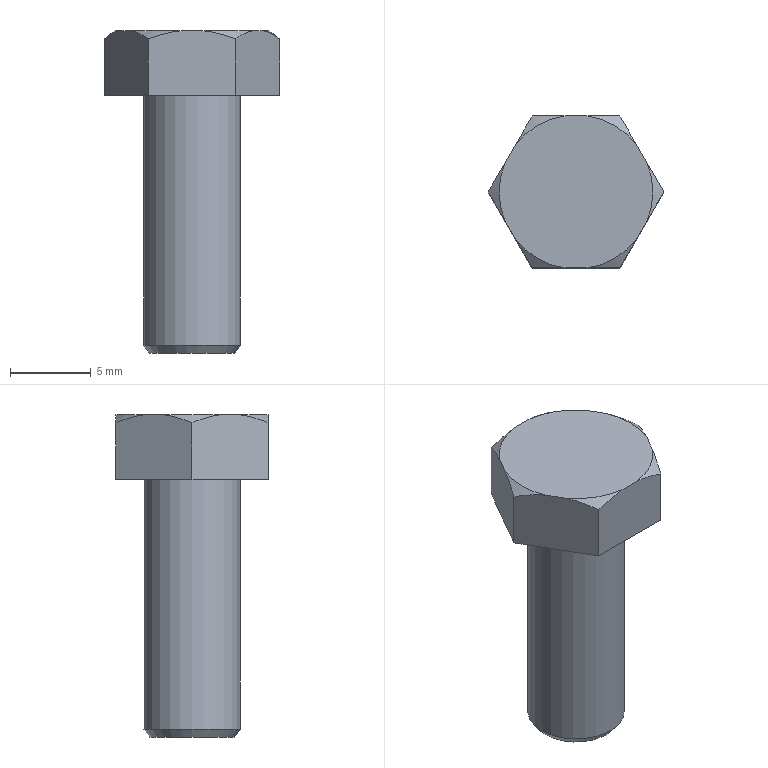Part | STEP file | GB5783-2000 bolt M6X16 | 1 solid | 17 faces | box 10.89 x 9.431 x 20 mm | volume 757.875 mm3 | plane 9 | cone 7 | cylinder 1 | commonest cylinder face diameters 6 x1
STEP:
#1=CARTESIAN_POINT('',(-2.625,0.,0.));
#2=VERTEX_POINT('',#1);
#3=CARTESIAN_POINT('',(0.,0.,0.));
#4=DIRECTION('',(0.,0.,-1.));
#5=DIRECTION('',(-1.,0.,0.));
#6=AXIS2_PLACEMENT_3D('',#3,#4,#5);
#7=CIRCLE('',#6,2.625);
#8=EDGE_CURVE('',#2,#2,#7,.T.);
#9=ORIENTED_EDGE('',*,*,#8,.T.);
#10=EDGE_LOOP('',(#9));
#11=FACE_OUTER_BOUND('',#10,.T.);
#12=CARTESIAN_POINT('',(0.,0.,0.));
#13=DIRECTION('',(0.,0.,1.));
#14=DIRECTION('',(1.,0.,0.));
#15=AXIS2_PLACEMENT_3D('',#12,#13,#14);
#16=PLANE('',#15);
#17=ADVANCED_FACE('',(#11),#16,.F.);
#18=CARTESIAN_POINT('',(-5.445,0.,16.));
#19=VERTEX_POINT('',#18);
#20=CARTESIAN_POINT('',(-2.722,-4.715,16.));
#21=VERTEX_POINT('',#20);
#22=CARTESIAN_POINT('',(-3.334,-3.657,16.));
#23=DIRECTION('',(0.5,-0.866,0.));
#24=VECTOR('',#23,1000.);
#25=LINE('',#22,#24);
#26=EDGE_CURVE('',#19,#21,#25,.T.);
#27=ORIENTED_EDGE('',*,*,#26,.F.);
#28=CARTESIAN_POINT('',(-2.723,4.715,16.));
#29=VERTEX_POINT('',#28);
#30=CARTESIAN_POINT('',(-3.334,3.657,16.));
#31=DIRECTION('',(-0.5,-0.866,0.));
#32=VECTOR('',#31,1000.);
#33=LINE('',#30,#32);
#34=EDGE_CURVE('',#29,#19,#33,.T.);
#35=ORIENTED_EDGE('',*,*,#34,.F.);
#36=CARTESIAN_POINT('',(2.723,4.715,16.));
#37=VERTEX_POINT('',#36);
#38=CARTESIAN_POINT('',(3.,4.715,16.));
#39=DIRECTION('',(-1.,0.,0.));
#40=VECTOR('',#39,1000.);
#41=LINE('',#38,#40);
#42=EDGE_CURVE('',#37,#29,#41,.T.);
#43=ORIENTED_EDGE('',*,*,#42,.F.);
#44=CARTESIAN_POINT('',(5.445,0.,16.));
#45=VERTEX_POINT('',#44);
#46=CARTESIAN_POINT('',(4.834,1.059,16.));
#47=DIRECTION('',(-0.5,0.866,0.));
#48=VECTOR('',#47,1000.);
#49=LINE('',#46,#48);
#50=EDGE_CURVE('',#45,#37,#49,.T.);
#51=ORIENTED_EDGE('',*,*,#50,.F.);
#52=CARTESIAN_POINT('',(2.723,-4.715,16.));
#53=VERTEX_POINT('',#52);
#54=CARTESIAN_POINT('',(4.834,-1.059,16.));
#55=DIRECTION('',(0.5,0.866,0.));
#56=VECTOR('',#55,1000.);
#57=LINE('',#54,#56);
#58=EDGE_CURVE('',#53,#45,#57,.T.);
#59=ORIENTED_EDGE('',*,*,#58,.F.);
#60=CARTESIAN_POINT('',(3.,-4.715,16.));
#61=DIRECTION('',(1.,0.,0.));
#62=VECTOR('',#61,1000.);
#63=LINE('',#60,#62);
#64=EDGE_CURVE('',#21,#53,#63,.T.);
#65=ORIENTED_EDGE('',*,*,#64,.F.);
#66=EDGE_LOOP('',(#27,#35,#43,#51,#59,#65));
#67=FACE_OUTER_BOUND('',#66,.T.);
#68=CARTESIAN_POINT('',(-3.,0.,16.));
#69=VERTEX_POINT('',#68);
#70=CARTESIAN_POINT('',(0.,0.,16.));
#71=DIRECTION('',(0.,0.,-1.));
#72=DIRECTION('',(-1.,0.,0.));
#73=AXIS2_PLACEMENT_3D('',#70,#71,#72);
#74=CIRCLE('',#73,3.);
#75=EDGE_CURVE('',#69,#69,#74,.T.);
#76=ORIENTED_EDGE('',*,*,#75,.F.);
#77=EDGE_LOOP('',(#76));
#78=FACE_BOUND('',#77,.T.);
#79=CARTESIAN_POINT('',(3.,0.,16.));
#80=DIRECTION('',(0.,0.,1.));
#81=DIRECTION('',(1.,0.,0.));
#82=AXIS2_PLACEMENT_3D('',#79,#80,#81);
#83=PLANE('',#82);
#84=ADVANCED_FACE('',(#67,#78),#83,.F.);
#85=CARTESIAN_POINT('',(-3.,0.,0.5));
#86=VERTEX_POINT('',#85);
#87=CARTESIAN_POINT('',(0.,0.,0.5));
#88=DIRECTION('',(0.,0.,-1.));
#89=DIRECTION('',(-1.,0.,0.));
#90=AXIS2_PLACEMENT_3D('',#87,#88,#89);
#91=CIRCLE('',#90,3.);
#92=EDGE_CURVE('',#86,#86,#91,.T.);
#93=ORIENTED_EDGE('',*,*,#92,.F.);
#94=EDGE_LOOP('',(#93));
#95=FACE_OUTER_BOUND('',#94,.T.);
#96=ORIENTED_EDGE('',*,*,#75,.T.);
#97=EDGE_LOOP('',(#96));
#98=FACE_OUTER_BOUND('',#97,.T.);
#99=CARTESIAN_POINT('',(0.,0.,0.));
#100=DIRECTION('',(0.,0.,-1.));
#101=DIRECTION('',(-1.,0.,0.));
#102=AXIS2_PLACEMENT_3D('',#99,#100,#101);
#103=CYLINDRICAL_SURFACE('',#102,3.);
#104=ADVANCED_FACE('',(#95,#98),#103,.T.);
#105=ORIENTED_EDGE('',*,*,#8,.F.);
#106=EDGE_LOOP('',(#105));
#107=FACE_BOUND('',#106,.T.);
#108=ORIENTED_EDGE('',*,*,#92,.T.);
#109=EDGE_LOOP('',(#108));
#110=FACE_OUTER_BOUND('',#109,.T.);
#111=CARTESIAN_POINT('',(0.,0.,0.5));
#112=DIRECTION('',(0.,0.,1.));
#113=DIRECTION('',(1.,0.,0.));
#114=AXIS2_PLACEMENT_3D('',#111,#112,#113);
#115=CONICAL_SURFACE('',#114,3.,0.6435);
#116=ADVANCED_FACE('',(#107,#110),#115,.T.);
#117=CARTESIAN_POINT('',(-2.722,-4.715,19.5));
#118=VERTEX_POINT('',#117);
#119=CARTESIAN_POINT('',(-2.722,-4.715,20.));
#120=DIRECTION('',(0.,0.,-1.));
#121=VECTOR('',#120,1000.);
#122=LINE('',#119,#121);
#123=EDGE_CURVE('',#118,#21,#122,.T.);
#124=ORIENTED_EDGE('',*,*,#123,.F.);
#125=CARTESIAN_POINT('',(-3.743,-2.947,20.));
#126=VERTEX_POINT('',#125);
#127=CARTESIAN_POINT('',(-2.722,-4.715,19.5));
#128=CARTESIAN_POINT('',(-3.054,-4.141,19.744));
#129=CARTESIAN_POINT('',(-3.393,-3.555,19.926));
#130=CARTESIAN_POINT('',(-3.743,-2.947,20.));
#131=B_SPLINE_CURVE_WITH_KNOTS('',3,(#127,#128,#129,#130),.UNSPECIFIED.,.F.,.F.,(4,4),(0.004241,0.00635),.UNSPECIFIED.);
#132=EDGE_CURVE('',#118,#126,#131,.T.);
#133=ORIENTED_EDGE('',*,*,#132,.T.);
#134=CARTESIAN_POINT('',(-4.424,-1.768,20.));
#135=VERTEX_POINT('',#134);
#136=CARTESIAN_POINT('',(-2.722,-4.715,20.));
#137=DIRECTION('',(-0.5,0.866,0.));
#138=VECTOR('',#137,1000.);
#139=LINE('',#136,#138);
#140=EDGE_CURVE('',#126,#135,#139,.T.);
#141=ORIENTED_EDGE('',*,*,#140,.T.);
#142=CARTESIAN_POINT('',(-5.445,0.,19.5));
#143=VERTEX_POINT('',#142);
#144=CARTESIAN_POINT('',(-4.424,-1.768,20.));
#145=CARTESIAN_POINT('',(-4.598,-1.467,19.964));
#146=CARTESIAN_POINT('',(-4.77,-1.169,19.9));
#147=CARTESIAN_POINT('',(-5.11,-0.5794,19.729));
#148=CARTESIAN_POINT('',(-5.28,-0.2861,19.621));
#149=CARTESIAN_POINT('',(-5.445,0.,19.5));
#150=B_SPLINE_CURVE_WITH_KNOTS('',3,(#144,#145,#146,#147,#148,#149),.UNSPECIFIED.,.F.,.F.,(4,2,4),(0.00771,0.008765,0.00982),.UNSPECIFIED.);
#151=EDGE_CURVE('',#135,#143,#150,.T.);
#152=ORIENTED_EDGE('',*,*,#151,.T.);
#153=CARTESIAN_POINT('',(-5.445,0.,20.));
#154=DIRECTION('',(0.,0.,-1.));
#155=VECTOR('',#154,1000.);
#156=LINE('',#153,#155);
#157=EDGE_CURVE('',#143,#19,#156,.T.);
#158=ORIENTED_EDGE('',*,*,#157,.T.);
#159=ORIENTED_EDGE('',*,*,#26,.T.);
#160=EDGE_LOOP('',(#124,#133,#141,#152,#158,#159));
#161=FACE_OUTER_BOUND('',#160,.T.);
#162=CARTESIAN_POINT('',(-2.722,-4.715,20.));
#163=DIRECTION('',(-0.866,-0.5,0.));
#164=DIRECTION('',(0.5,-0.866,0.));
#165=AXIS2_PLACEMENT_3D('',#162,#163,#164);
#166=PLANE('',#165);
#167=ADVANCED_FACE('',(#161),#166,.T.);
#168=CARTESIAN_POINT('',(2.722,-4.715,19.5));
#169=VERTEX_POINT('',#168);
#170=CARTESIAN_POINT('',(2.723,-4.715,20.));
#171=DIRECTION('',(0.,0.,-1.));
#172=VECTOR('',#171,1000.);
#173=LINE('',#170,#172);
#174=EDGE_CURVE('',#169,#53,#173,.T.);
#175=ORIENTED_EDGE('',*,*,#174,.F.);
#176=CARTESIAN_POINT('',(0.6816,-4.715,20.));
#177=VERTEX_POINT('',#176);
#178=CARTESIAN_POINT('',(2.722,-4.715,19.5));
#179=CARTESIAN_POINT('',(2.392,-4.715,19.621));
#180=CARTESIAN_POINT('',(2.054,-4.715,19.729));
#181=CARTESIAN_POINT('',(1.373,-4.715,19.9));
#182=CARTESIAN_POINT('',(1.029,-4.715,19.963));
#183=CARTESIAN_POINT('',(0.6816,-4.715,20.));
#184=B_SPLINE_CURVE_WITH_KNOTS('',3,(#178,#179,#180,#181,#182,#183),.UNSPECIFIED.,.F.,.F.,(4,2,4),(0.003653,0.004704,0.005755),.UNSPECIFIED.);
#185=EDGE_CURVE('',#169,#177,#184,.T.);
#186=ORIENTED_EDGE('',*,*,#185,.T.);
#187=CARTESIAN_POINT('',(-0.6816,-4.715,20.));
#188=VERTEX_POINT('',#187);
#189=CARTESIAN_POINT('',(2.723,-4.715,20.));
#190=DIRECTION('',(-1.,0.,0.));
#191=VECTOR('',#190,1000.);
#192=LINE('',#189,#191);
#193=EDGE_CURVE('',#177,#188,#192,.T.);
#194=ORIENTED_EDGE('',*,*,#193,.T.);
#195=CARTESIAN_POINT('',(-0.6816,-4.715,20.));
#196=CARTESIAN_POINT('',(-1.382,-4.715,19.926));
#197=CARTESIAN_POINT('',(-2.059,-4.715,19.744));
#198=CARTESIAN_POINT('',(-2.722,-4.715,19.5));
#199=B_SPLINE_CURVE_WITH_KNOTS('',3,(#195,#196,#197,#198),.UNSPECIFIED.,.F.,.F.,(4,4),(0.007114,0.009216),.UNSPECIFIED.);
#200=EDGE_CURVE('',#188,#118,#199,.T.);
#201=ORIENTED_EDGE('',*,*,#200,.T.);
#202=ORIENTED_EDGE('',*,*,#123,.T.);
#203=ORIENTED_EDGE('',*,*,#64,.T.);
#204=EDGE_LOOP('',(#175,#186,#194,#201,#202,#203));
#205=FACE_OUTER_BOUND('',#204,.T.);
#206=CARTESIAN_POINT('',(2.723,-4.715,20.));
#207=DIRECTION('',(0.,-1.,0.));
#208=DIRECTION('',(1.,0.,0.));
#209=AXIS2_PLACEMENT_3D('',#206,#207,#208);
#210=PLANE('',#209);
#211=ADVANCED_FACE('',(#205),#210,.T.);
#212=CARTESIAN_POINT('',(5.445,0.,19.5));
#213=VERTEX_POINT('',#212);
#214=CARTESIAN_POINT('',(5.445,0.,20.));
#215=DIRECTION('',(0.,0.,-1.));
#216=VECTOR('',#215,1000.);
#217=LINE('',#214,#216);
#218=EDGE_CURVE('',#213,#45,#217,.T.);
#219=ORIENTED_EDGE('',*,*,#218,.F.);
#220=CARTESIAN_POINT('',(4.424,-1.768,20.));
#221=VERTEX_POINT('',#220);
#222=CARTESIAN_POINT('',(5.445,0.,19.5));
#223=CARTESIAN_POINT('',(5.113,-0.5746,19.744));
#224=CARTESIAN_POINT('',(4.775,-1.161,19.926));
#225=CARTESIAN_POINT('',(4.424,-1.768,20.));
#226=B_SPLINE_CURVE_WITH_KNOTS('',3,(#222,#223,#224,#225),.UNSPECIFIED.,.F.,.F.,(4,4),(0.004241,0.00635),.UNSPECIFIED.);
#227=EDGE_CURVE('',#213,#221,#226,.T.);
#228=ORIENTED_EDGE('',*,*,#227,.T.);
#229=CARTESIAN_POINT('',(3.743,-2.947,20.));
#230=VERTEX_POINT('',#229);
#231=CARTESIAN_POINT('',(5.445,0.,20.));
#232=DIRECTION('',(-0.5,-0.866,0.));
#233=VECTOR('',#232,1000.);
#234=LINE('',#231,#233);
#235=EDGE_CURVE('',#221,#230,#234,.T.);
#236=ORIENTED_EDGE('',*,*,#235,.T.);
#237=CARTESIAN_POINT('',(3.743,-2.947,20.));
#238=CARTESIAN_POINT('',(3.569,-3.248,19.964));
#239=CARTESIAN_POINT('',(3.398,-3.546,19.9));
#240=CARTESIAN_POINT('',(3.057,-4.136,19.729));
#241=CARTESIAN_POINT('',(2.888,-4.429,19.621));
#242=CARTESIAN_POINT('',(2.722,-4.715,19.5));
#243=B_SPLINE_CURVE_WITH_KNOTS('',3,(#237,#238,#239,#240,#241,#242),.UNSPECIFIED.,.F.,.F.,(4,2,4),(0.007711,0.008765,0.00982),.UNSPECIFIED.);
#244=EDGE_CURVE('',#230,#169,#243,.T.);
#245=ORIENTED_EDGE('',*,*,#244,.T.);
#246=ORIENTED_EDGE('',*,*,#174,.T.);
#247=ORIENTED_EDGE('',*,*,#58,.T.);
#248=EDGE_LOOP('',(#219,#228,#236,#245,#246,#247));
#249=FACE_OUTER_BOUND('',#248,.T.);
#250=CARTESIAN_POINT('',(5.445,0.,20.));
#251=DIRECTION('',(0.866,-0.5,0.));
#252=DIRECTION('',(0.5,0.866,0.));
#253=AXIS2_PLACEMENT_3D('',#250,#251,#252);
#254=PLANE('',#253);
#255=ADVANCED_FACE('',(#249),#254,.T.);
#256=CARTESIAN_POINT('',(2.723,4.715,19.5));
#257=VERTEX_POINT('',#256);
#258=CARTESIAN_POINT('',(2.723,4.715,20.));
#259=DIRECTION('',(0.,0.,-1.));
#260=VECTOR('',#259,1000.);
#261=LINE('',#258,#260);
#262=EDGE_CURVE('',#257,#37,#261,.T.);
#263=ORIENTED_EDGE('',*,*,#262,.F.);
#264=CARTESIAN_POINT('',(3.743,2.947,20.));
#265=VERTEX_POINT('',#264);
#266=CARTESIAN_POINT('',(2.723,4.715,19.5));
#267=CARTESIAN_POINT('',(3.054,4.141,19.744));
#268=CARTESIAN_POINT('',(3.393,3.555,19.926));
#269=CARTESIAN_POINT('',(3.743,2.947,20.));
#270=B_SPLINE_CURVE_WITH_KNOTS('',3,(#266,#267,#268,#269),.UNSPECIFIED.,.F.,.F.,(4,4),(0.004241,0.00635),.UNSPECIFIED.);
#271=EDGE_CURVE('',#257,#265,#270,.T.);
#272=ORIENTED_EDGE('',*,*,#271,.T.);
#273=CARTESIAN_POINT('',(4.424,1.768,20.));
#274=VERTEX_POINT('',#273);
#275=CARTESIAN_POINT('',(2.723,4.715,20.));
#276=DIRECTION('',(0.5,-0.866,0.));
#277=VECTOR('',#276,1000.);
#278=LINE('',#275,#277);
#279=EDGE_CURVE('',#265,#274,#278,.T.);
#280=ORIENTED_EDGE('',*,*,#279,.T.);
#281=CARTESIAN_POINT('',(4.424,1.768,20.));
#282=CARTESIAN_POINT('',(4.598,1.467,19.964));
#283=CARTESIAN_POINT('',(4.77,1.169,19.9));
#284=CARTESIAN_POINT('',(5.11,0.5794,19.729));
#285=CARTESIAN_POINT('',(5.28,0.2861,19.621));
#286=CARTESIAN_POINT('',(5.445,0.,19.5));
#287=B_SPLINE_CURVE_WITH_KNOTS('',3,(#281,#282,#283,#284,#285,#286),.UNSPECIFIED.,.F.,.F.,(4,2,4),(0.00771,0.008765,0.00982),.UNSPECIFIED.);
#288=EDGE_CURVE('',#274,#213,#287,.T.);
#289=ORIENTED_EDGE('',*,*,#288,.T.);
#290=ORIENTED_EDGE('',*,*,#218,.T.);
#291=ORIENTED_EDGE('',*,*,#50,.T.);
#292=EDGE_LOOP('',(#263,#272,#280,#289,#290,#291));
#293=FACE_OUTER_BOUND('',#292,.T.);
#294=CARTESIAN_POINT('',(2.723,4.715,20.));
#295=DIRECTION('',(0.866,0.5,0.));
#296=DIRECTION('',(-0.5,0.866,0.));
#297=AXIS2_PLACEMENT_3D('',#294,#295,#296);
#298=PLANE('',#297);
#299=ADVANCED_FACE('',(#293),#298,.T.);
#300=CARTESIAN_POINT('',(-2.723,4.715,19.5));
#301=VERTEX_POINT('',#300);
#302=CARTESIAN_POINT('',(-2.723,4.715,20.));
#303=DIRECTION('',(0.,0.,-1.));
#304=VECTOR('',#303,1000.);
#305=LINE('',#302,#304);
#306=EDGE_CURVE('',#301,#29,#305,.T.);
#307=ORIENTED_EDGE('',*,*,#306,.F.);
#308=CARTESIAN_POINT('',(-0.6816,4.715,20.));
#309=VERTEX_POINT('',#308);
#310=CARTESIAN_POINT('',(-2.723,4.715,19.5));
#311=CARTESIAN_POINT('',(-2.392,4.715,19.621));
#312=CARTESIAN_POINT('',(-2.054,4.715,19.729));
#313=CARTESIAN_POINT('',(-1.373,4.715,19.9));
#314=CARTESIAN_POINT('',(-1.029,4.715,19.963));
#315=CARTESIAN_POINT('',(-0.6816,4.715,20.));
#316=B_SPLINE_CURVE_WITH_KNOTS('',3,(#310,#311,#312,#313,#314,#315),.UNSPECIFIED.,.F.,.F.,(4,2,4),(0.003653,0.004704,0.005755),.UNSPECIFIED.);
#317=EDGE_CURVE('',#301,#309,#316,.T.);
#318=ORIENTED_EDGE('',*,*,#317,.T.);
#319=CARTESIAN_POINT('',(0.6816,4.715,20.));
#320=VERTEX_POINT('',#319);
#321=CARTESIAN_POINT('',(-2.723,4.715,20.));
#322=DIRECTION('',(1.,0.,0.));
#323=VECTOR('',#322,1000.);
#324=LINE('',#321,#323);
#325=EDGE_CURVE('',#309,#320,#324,.T.);
#326=ORIENTED_EDGE('',*,*,#325,.T.);
#327=CARTESIAN_POINT('',(0.6816,4.715,20.));
#328=CARTESIAN_POINT('',(1.382,4.715,19.926));
#329=CARTESIAN_POINT('',(2.059,4.715,19.744));
#330=CARTESIAN_POINT('',(2.723,4.715,19.5));
#331=B_SPLINE_CURVE_WITH_KNOTS('',3,(#327,#328,#329,#330),.UNSPECIFIED.,.F.,.F.,(4,4),(0.007114,0.009216),.UNSPECIFIED.);
#332=EDGE_CURVE('',#320,#257,#331,.T.);
#333=ORIENTED_EDGE('',*,*,#332,.T.);
#334=ORIENTED_EDGE('',*,*,#262,.T.);
#335=ORIENTED_EDGE('',*,*,#42,.T.);
#336=EDGE_LOOP('',(#307,#318,#326,#333,#334,#335));
#337=FACE_OUTER_BOUND('',#336,.T.);
#338=CARTESIAN_POINT('',(-2.723,4.715,20.));
#339=DIRECTION('',(0.,1.,0.));
#340=DIRECTION('',(0.,0.,1.));
#341=AXIS2_PLACEMENT_3D('',#338,#339,#340);
#342=PLANE('',#341);
#343=ADVANCED_FACE('',(#337),#342,.T.);
#344=ORIENTED_EDGE('',*,*,#157,.F.);
#345=CARTESIAN_POINT('',(-4.424,1.768,20.));
#346=VERTEX_POINT('',#345);
#347=CARTESIAN_POINT('',(-5.445,0.,19.5));
#348=CARTESIAN_POINT('',(-5.113,0.5746,19.744));
#349=CARTESIAN_POINT('',(-4.775,1.161,19.926));
#350=CARTESIAN_POINT('',(-4.424,1.768,20.));
#351=B_SPLINE_CURVE_WITH_KNOTS('',3,(#347,#348,#349,#350),.UNSPECIFIED.,.F.,.F.,(4,4),(0.004241,0.00635),.UNSPECIFIED.);
#352=EDGE_CURVE('',#143,#346,#351,.T.);
#353=ORIENTED_EDGE('',*,*,#352,.T.);
#354=CARTESIAN_POINT('',(-3.743,2.947,20.));
#355=VERTEX_POINT('',#354);
#356=CARTESIAN_POINT('',(-5.445,0.,20.));
#357=DIRECTION('',(0.5,0.866,0.));
#358=VECTOR('',#357,1000.);
#359=LINE('',#356,#358);
#360=EDGE_CURVE('',#346,#355,#359,.T.);
#361=ORIENTED_EDGE('',*,*,#360,.T.);
#362=CARTESIAN_POINT('',(-3.743,2.947,20.));
#363=CARTESIAN_POINT('',(-3.569,3.248,19.964));
#364=CARTESIAN_POINT('',(-3.398,3.546,19.9));
#365=CARTESIAN_POINT('',(-3.057,4.136,19.729));
#366=CARTESIAN_POINT('',(-2.888,4.429,19.621));
#367=CARTESIAN_POINT('',(-2.723,4.715,19.5));
#368=B_SPLINE_CURVE_WITH_KNOTS('',3,(#362,#363,#364,#365,#366,#367),.UNSPECIFIED.,.F.,.F.,(4,2,4),(0.007711,0.008765,0.00982),.UNSPECIFIED.);
#369=EDGE_CURVE('',#355,#301,#368,.T.);
#370=ORIENTED_EDGE('',*,*,#369,.T.);
#371=ORIENTED_EDGE('',*,*,#306,.T.);
#372=ORIENTED_EDGE('',*,*,#34,.T.);
#373=EDGE_LOOP('',(#344,#353,#361,#370,#371,#372));
#374=FACE_OUTER_BOUND('',#373,.T.);
#375=CARTESIAN_POINT('',(-5.445,0.,20.));
#376=DIRECTION('',(-0.866,0.5,0.));
#377=DIRECTION('',(-0.5,-0.866,0.));
#378=AXIS2_PLACEMENT_3D('',#375,#376,#377);
#379=PLANE('',#378);
#380=ADVANCED_FACE('',(#374),#379,.T.);
#381=ORIENTED_EDGE('',*,*,#151,.F.);
#382=CARTESIAN_POINT('',(0.,0.,20.));
#383=DIRECTION('',(0.,0.,-1.));
#384=DIRECTION('',(-1.,0.,0.));
#385=AXIS2_PLACEMENT_3D('',#382,#383,#384);
#386=CIRCLE('',#385,4.764);
#387=EDGE_CURVE('',#135,#346,#386,.T.);
#388=ORIENTED_EDGE('',*,*,#387,.T.);
#389=ORIENTED_EDGE('',*,*,#352,.F.);
#390=EDGE_LOOP('',(#381,#388,#389));
#391=FACE_OUTER_BOUND('',#390,.T.);
#392=CARTESIAN_POINT('',(0.,0.,20.));
#393=DIRECTION('',(0.,0.,-1.));
#394=DIRECTION('',(-1.,0.,0.));
#395=AXIS2_PLACEMENT_3D('',#392,#393,#394);
#396=CONICAL_SURFACE('',#395,4.764,0.9372);
#397=ADVANCED_FACE('',(#391),#396,.T.);
#398=ORIENTED_EDGE('',*,*,#317,.F.);
#399=ORIENTED_EDGE('',*,*,#369,.F.);
#400=CARTESIAN_POINT('',(0.,0.,20.));
#401=DIRECTION('',(0.,0.,-1.));
#402=DIRECTION('',(-1.,0.,0.));
#403=AXIS2_PLACEMENT_3D('',#400,#401,#402);
#404=CIRCLE('',#403,4.764);
#405=EDGE_CURVE('',#355,#309,#404,.T.);
#406=ORIENTED_EDGE('',*,*,#405,.T.);
#407=EDGE_LOOP('',(#398,#399,#406));
#408=FACE_OUTER_BOUND('',#407,.T.);
#409=CARTESIAN_POINT('',(0.,0.,20.));
#410=DIRECTION('',(0.,0.,-1.));
#411=DIRECTION('',(-1.,0.,0.));
#412=AXIS2_PLACEMENT_3D('',#409,#410,#411);
#413=CONICAL_SURFACE('',#412,4.764,0.9372);
#414=ADVANCED_FACE('',(#408),#413,.T.);
#415=ORIENTED_EDGE('',*,*,#271,.F.);
#416=ORIENTED_EDGE('',*,*,#332,.F.);
#417=CARTESIAN_POINT('',(0.,0.,20.));
#418=DIRECTION('',(0.,0.,-1.));
#419=DIRECTION('',(-1.,0.,0.));
#420=AXIS2_PLACEMENT_3D('',#417,#418,#419);
#421=CIRCLE('',#420,4.764);
#422=EDGE_CURVE('',#320,#265,#421,.T.);
#423=ORIENTED_EDGE('',*,*,#422,.T.);
#424=EDGE_LOOP('',(#415,#416,#423));
#425=FACE_OUTER_BOUND('',#424,.T.);
#426=CARTESIAN_POINT('',(0.,0.,20.));
#427=DIRECTION('',(0.,0.,-1.));
#428=DIRECTION('',(-1.,0.,0.));
#429=AXIS2_PLACEMENT_3D('',#426,#427,#428);
#430=CONICAL_SURFACE('',#429,4.764,0.9372);
#431=ADVANCED_FACE('',(#425),#430,.T.);
#432=ORIENTED_EDGE('',*,*,#227,.F.);
#433=ORIENTED_EDGE('',*,*,#288,.F.);
#434=CARTESIAN_POINT('',(0.,0.,20.));
#435=DIRECTION('',(0.,0.,-1.));
#436=DIRECTION('',(-1.,0.,0.));
#437=AXIS2_PLACEMENT_3D('',#434,#435,#436);
#438=CIRCLE('',#437,4.764);
#439=EDGE_CURVE('',#274,#221,#438,.T.);
#440=ORIENTED_EDGE('',*,*,#439,.T.);
#441=EDGE_LOOP('',(#432,#433,#440));
#442=FACE_OUTER_BOUND('',#441,.T.);
#443=CARTESIAN_POINT('',(0.,0.,20.));
#444=DIRECTION('',(0.,0.,-1.));
#445=DIRECTION('',(-1.,0.,0.));
#446=AXIS2_PLACEMENT_3D('',#443,#444,#445);
#447=CONICAL_SURFACE('',#446,4.764,0.9372);
#448=ADVANCED_FACE('',(#442),#447,.T.);
#449=ORIENTED_EDGE('',*,*,#185,.F.);
#450=ORIENTED_EDGE('',*,*,#244,.F.);
#451=CARTESIAN_POINT('',(0.,0.,20.));
#452=DIRECTION('',(0.,0.,-1.));
#453=DIRECTION('',(-1.,0.,0.));
#454=AXIS2_PLACEMENT_3D('',#451,#452,#453);
#455=CIRCLE('',#454,4.764);
#456=EDGE_CURVE('',#230,#177,#455,.T.);
#457=ORIENTED_EDGE('',*,*,#456,.T.);
#458=EDGE_LOOP('',(#449,#450,#457));
#459=FACE_OUTER_BOUND('',#458,.T.);
#460=CARTESIAN_POINT('',(0.,0.,20.));
#461=DIRECTION('',(0.,0.,-1.));
#462=DIRECTION('',(-1.,0.,0.));
#463=AXIS2_PLACEMENT_3D('',#460,#461,#462);
#464=CONICAL_SURFACE('',#463,4.764,0.9372);
#465=ADVANCED_FACE('',(#459),#464,.T.);
#466=ORIENTED_EDGE('',*,*,#132,.F.);
#467=ORIENTED_EDGE('',*,*,#200,.F.);
#468=CARTESIAN_POINT('',(0.,0.,20.));
#469=DIRECTION('',(0.,0.,-1.));
#470=DIRECTION('',(-1.,0.,0.));
#471=AXIS2_PLACEMENT_3D('',#468,#469,#470);
#472=CIRCLE('',#471,4.764);
#473=EDGE_CURVE('',#188,#126,#472,.T.);
#474=ORIENTED_EDGE('',*,*,#473,.T.);
#475=EDGE_LOOP('',(#466,#467,#474));
#476=FACE_OUTER_BOUND('',#475,.T.);
#477=CARTESIAN_POINT('',(0.,0.,20.));
#478=DIRECTION('',(0.,0.,-1.));
#479=DIRECTION('',(-1.,0.,0.));
#480=AXIS2_PLACEMENT_3D('',#477,#478,#479);
#481=CONICAL_SURFACE('',#480,4.764,0.9372);
#482=ADVANCED_FACE('',(#476),#481,.T.);
#483=ORIENTED_EDGE('',*,*,#140,.F.);
#484=ORIENTED_EDGE('',*,*,#473,.F.);
#485=ORIENTED_EDGE('',*,*,#193,.F.);
#486=ORIENTED_EDGE('',*,*,#456,.F.);
#487=ORIENTED_EDGE('',*,*,#235,.F.);
#488=ORIENTED_EDGE('',*,*,#439,.F.);
#489=ORIENTED_EDGE('',*,*,#279,.F.);
#490=ORIENTED_EDGE('',*,*,#422,.F.);
#491=ORIENTED_EDGE('',*,*,#325,.F.);
#492=ORIENTED_EDGE('',*,*,#405,.F.);
#493=ORIENTED_EDGE('',*,*,#360,.F.);
#494=ORIENTED_EDGE('',*,*,#387,.F.);
#495=EDGE_LOOP('',(#483,#484,#485,#486,#487,#488,#489,#490,#491,#492,#493,#494));
#496=FACE_OUTER_BOUND('',#495,.T.);
#497=CARTESIAN_POINT('',(4.764,0.,20.));
#498=DIRECTION('',(0.,0.,-1.));
#499=DIRECTION('',(-1.,0.,0.));
#500=AXIS2_PLACEMENT_3D('',#497,#498,#499);
#501=PLANE('',#500);
#502=ADVANCED_FACE('',(#496),#501,.F.);
#503=CLOSED_SHELL('',(#17,#84,#104,#116,#167,#211,#255,#299,#343,#380,#397,#414,#431,#448,#465,#482,#502));
#504=MANIFOLD_SOLID_BREP('',#503);
#505=CARTESIAN_POINT('',(0.,0.,0.));
#506=DIRECTION('',(0.,0.,1.));
#507=DIRECTION('',(1.,0.,0.));
#508=AXIS2_PLACEMENT_3D('',#505,#506,#507);
#509=(LENGTH_UNIT()NAMED_UNIT(*)SI_UNIT(.MILLI.,.METRE.));
#510=UNCERTAINTY_MEASURE_WITH_UNIT(LENGTH_MEASURE(0.00001),#509,'','');
#511=(NAMED_UNIT(*)PLANE_ANGLE_UNIT()SI_UNIT($,.RADIAN.));
#512=(NAMED_UNIT(*)SI_UNIT($,.STERADIAN.)SOLID_ANGLE_UNIT());
#513=(GEOMETRIC_REPRESENTATION_CONTEXT(3)GLOBAL_UNCERTAINTY_ASSIGNED_CONTEXT((#510))GLOBAL_UNIT_ASSIGNED_CONTEXT((#509,#511,#512))REPRESENTATION_CONTEXT('',''));
#514=ADVANCED_BREP_SHAPE_REPRESENTATION('',(#504,#508),#513);